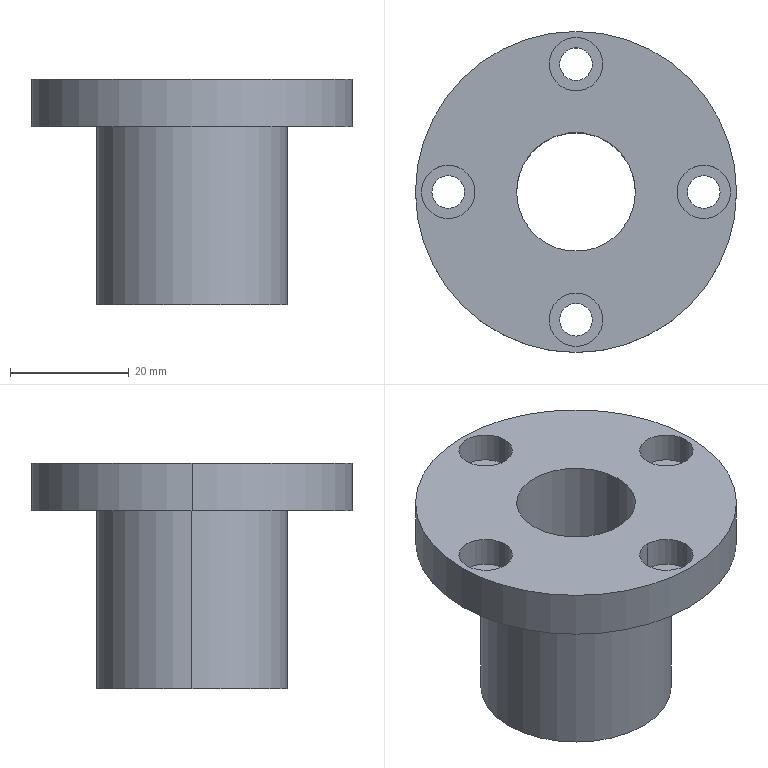Part | STEP file | LMF01-d20-steel outer graphite inner- | 1 solid | 29 faces | box 54 x 54 x 38 mm | volume 28938 mm3 | cylinder 22 | plane 7 | commonest cylinder face diameters 5.5 x8 9 x8 20 x2 32 x2 54 x2